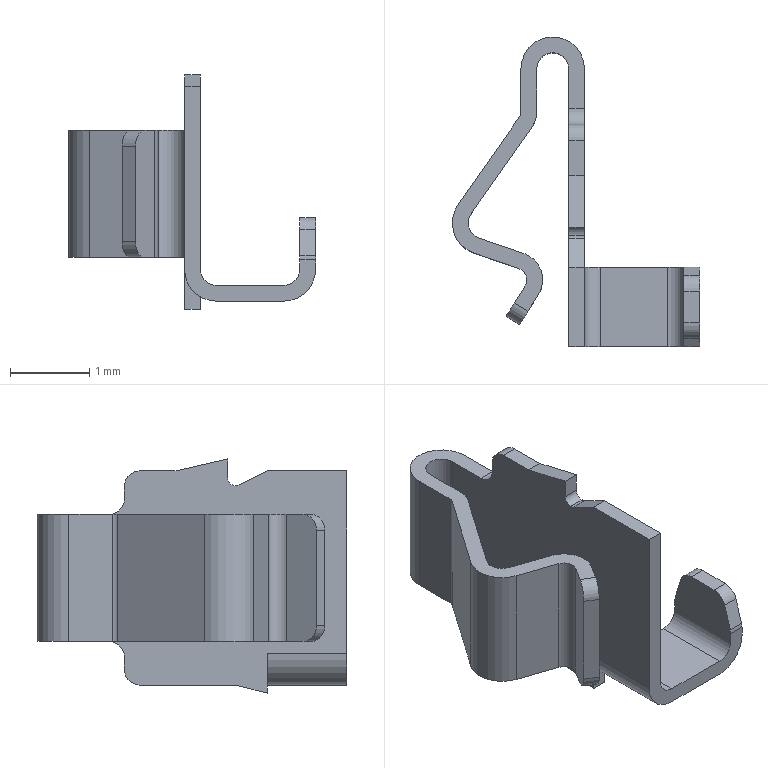Part | Creo | 1 solid | 57 faces | box 3.115 x 3.9 x 2.95 mm | volume 3.733 mm3 | plane 32 | cylinder 25 | commonest cylinder face diameters 0.4 x15 0.8 x4 0.2 x3 0.3 x1 0.6 x1 0.7 x1